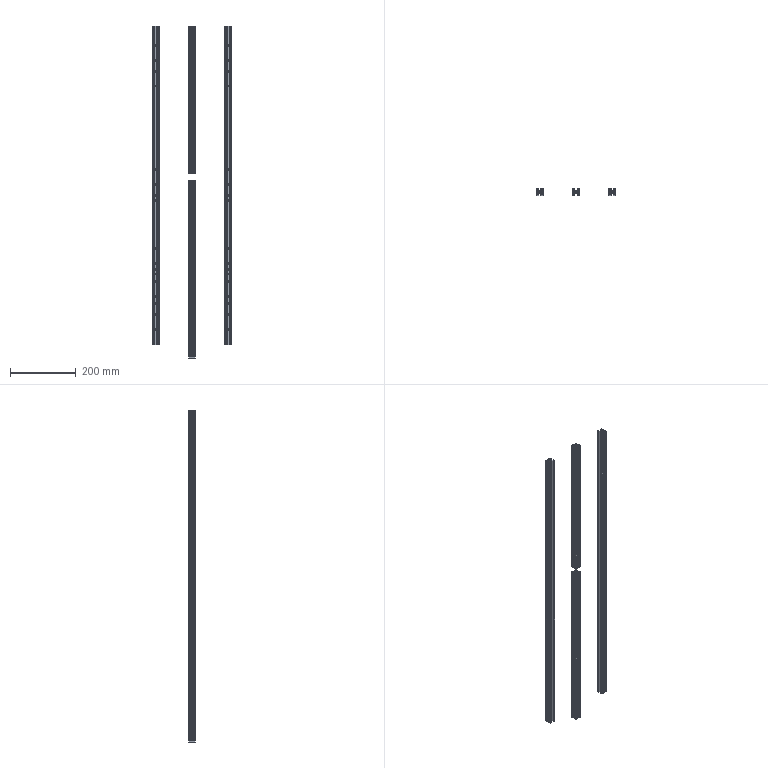Part | SolidWorks | features BaseBody 4 | 4 solids | 663 faces | box 240 x 20 x 1010 mm | volume 485681 mm3 | cylinder 414 | plane 249 | commonest cylinder face diameters 3 x214 5 x140 5.2 x36 4.2 x24